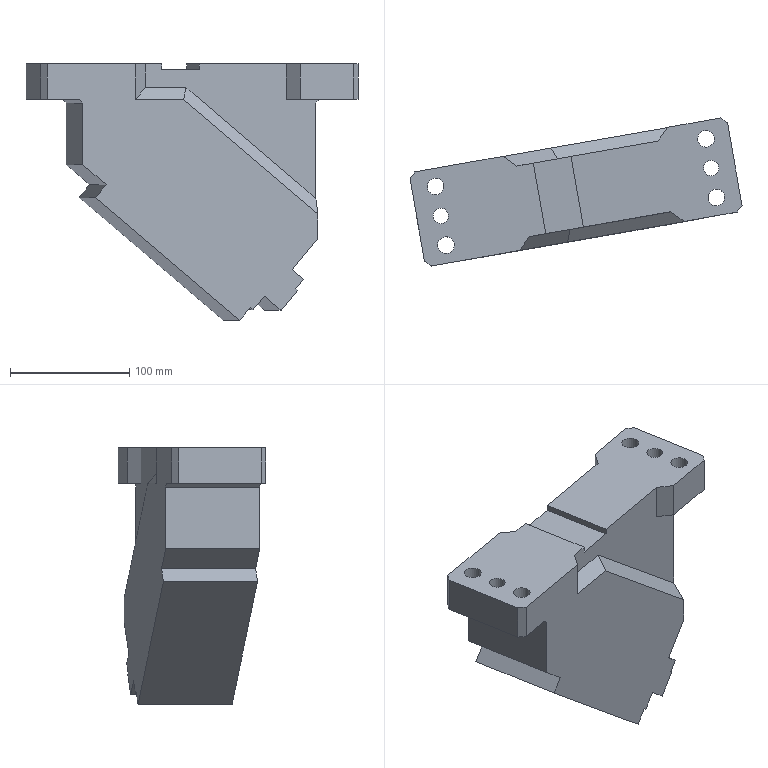Part | NX | features solid 2 | 1 solid | 57 faces | box 278.053 x 123.933 x 214.945 mm | volume 2645930 mm3 | plane 47 | cylinder 10 | commonest cylinder face diameters 14 x4 20 x4 13 x2